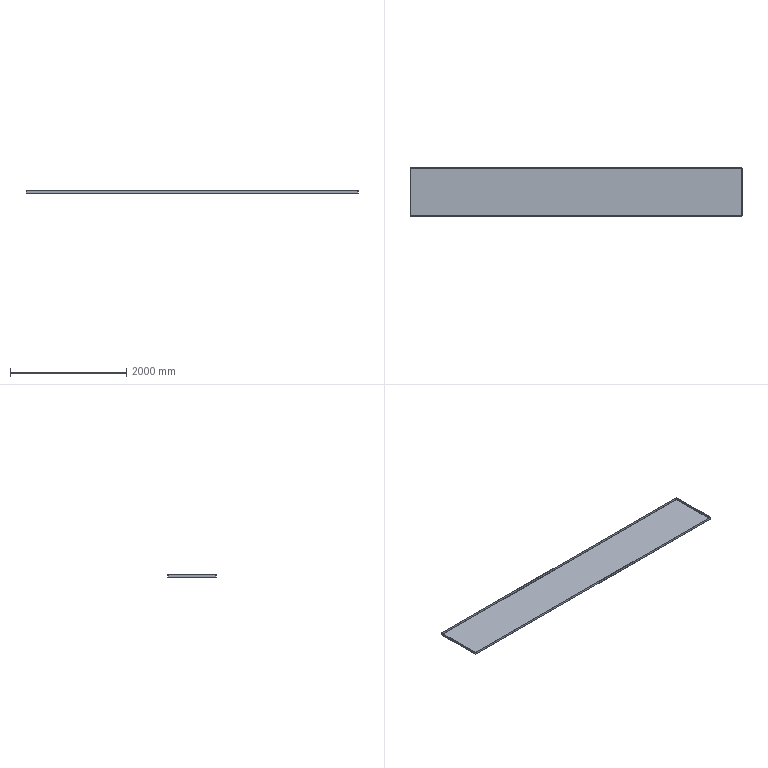Part | SolidWorks | features EdgeFlange 1, FlatPattern 1, SMBaseFlange 1, SheetMetal 1 | 1 solid | 38 faces | box 5700 x 825 x 40 mm | volume 10375674 mm3 | plane 22 | spline 8 | cylinder 8 | commonest cylinder face diameters 1.473 x4 5.473 x4
STEP:
#1=CARTESIAN_POINT('',(2847.263,409.763,-2.));
#2=VERTEX_POINT('',#1);
#3=CARTESIAN_POINT('',(2847.263,-409.763,-2.));
#4=VERTEX_POINT('',#3);
#5=CARTESIAN_POINT('',(2847.263,409.793,-2.));
#6=DIRECTION('',(0.,-1.,0.));
#7=VECTOR('',#6,1000.);
#8=LINE('',#5,#7);
#9=EDGE_CURVE('',#2,#4,#8,.T.);
#10=ORIENTED_EDGE('',*,*,#9,.T.);
#11=CARTESIAN_POINT('',(-2847.263,-409.763,-2.));
#12=VERTEX_POINT('',#11);
#13=CARTESIAN_POINT('',(2847.293,-409.763,-2.));
#14=DIRECTION('',(-1.,0.,0.));
#15=VECTOR('',#14,1000.);
#16=LINE('',#13,#15);
#17=EDGE_CURVE('',#4,#12,#16,.T.);
#18=ORIENTED_EDGE('',*,*,#17,.T.);
#19=CARTESIAN_POINT('',(-2847.263,409.763,-2.));
#20=VERTEX_POINT('',#19);
#21=CARTESIAN_POINT('',(-2847.263,-409.793,-2.));
#22=DIRECTION('',(0.,1.,0.));
#23=VECTOR('',#22,1000.);
#24=LINE('',#21,#23);
#25=EDGE_CURVE('',#12,#20,#24,.T.);
#26=ORIENTED_EDGE('',*,*,#25,.T.);
#27=CARTESIAN_POINT('',(-2847.293,409.763,-2.));
#28=DIRECTION('',(1.,0.,0.));
#29=VECTOR('',#28,1000.);
#30=LINE('',#27,#29);
#31=EDGE_CURVE('',#20,#2,#30,.T.);
#32=ORIENTED_EDGE('',*,*,#31,.T.);
#33=EDGE_LOOP('',(#10,#18,#26,#32));
#34=FACE_OUTER_BOUND('',#33,.T.);
#35=CARTESIAN_POINT('',(0.,0.,-2.));
#36=DIRECTION('',(0.,0.,-1.));
#37=DIRECTION('',(-1.,0.,0.));
#38=AXIS2_PLACEMENT_3D('',#35,#36,#37);
#39=PLANE('',#38);
#40=ADVANCED_FACE('',(#34),#39,.T.);
#41=CARTESIAN_POINT('',(2847.263,-409.763,0.));
#42=VERTEX_POINT('',#41);
#43=CARTESIAN_POINT('',(-2847.263,-409.763,0.));
#44=VERTEX_POINT('',#43);
#45=CARTESIAN_POINT('',(2847.293,-409.763,0.));
#46=DIRECTION('',(-1.,0.,0.));
#47=VECTOR('',#46,1000.);
#48=LINE('',#45,#47);
#49=EDGE_CURVE('',#42,#44,#48,.T.);
#50=ORIENTED_EDGE('',*,*,#49,.F.);
#51=CARTESIAN_POINT('',(2847.263,409.763,0.));
#52=VERTEX_POINT('',#51);
#53=CARTESIAN_POINT('',(2847.263,409.793,0.));
#54=DIRECTION('',(0.,-1.,0.));
#55=VECTOR('',#54,1000.);
#56=LINE('',#53,#55);
#57=EDGE_CURVE('',#52,#42,#56,.T.);
#58=ORIENTED_EDGE('',*,*,#57,.F.);
#59=CARTESIAN_POINT('',(-2847.263,409.763,0.));
#60=VERTEX_POINT('',#59);
#61=CARTESIAN_POINT('',(-2847.293,409.763,0.));
#62=DIRECTION('',(1.,0.,0.));
#63=VECTOR('',#62,1000.);
#64=LINE('',#61,#63);
#65=EDGE_CURVE('',#60,#52,#64,.T.);
#66=ORIENTED_EDGE('',*,*,#65,.F.);
#67=CARTESIAN_POINT('',(-2847.263,-409.793,0.));
#68=DIRECTION('',(0.,1.,0.));
#69=VECTOR('',#68,1000.);
#70=LINE('',#67,#69);
#71=EDGE_CURVE('',#44,#60,#70,.T.);
#72=ORIENTED_EDGE('',*,*,#71,.F.);
#73=EDGE_LOOP('',(#50,#58,#66,#72));
#74=FACE_OUTER_BOUND('',#73,.T.);
#75=CARTESIAN_POINT('',(0.,0.,0.));
#76=DIRECTION('',(0.,0.,-1.));
#77=DIRECTION('',(-1.,0.,0.));
#78=AXIS2_PLACEMENT_3D('',#75,#76,#77);
#79=PLANE('',#78);
#80=ADVANCED_FACE('',(#74),#79,.F.);
#81=CARTESIAN_POINT('',(2847.293,412.5,0.7366));
#82=VERTEX_POINT('',#81);
#83=CARTESIAN_POINT('',(2847.293,410.5,0.7366));
#84=VERTEX_POINT('',#83);
#85=CARTESIAN_POINT('',(2847.293,410.5,0.7366));
#86=DIRECTION('',(0.,-1.,0.));
#87=VECTOR('',#86,1000.);
#88=LINE('',#85,#87);
#89=EDGE_CURVE('',#82,#84,#88,.T.);
#90=ORIENTED_EDGE('',*,*,#89,.T.);
#91=CARTESIAN_POINT('',(2847.263,409.763,0.));
#92=CARTESIAN_POINT('',(2847.268,409.956,0.));
#93=CARTESIAN_POINT('',(2847.273,410.148,0.07939));
#94=CARTESIAN_POINT('',(2847.283,410.421,0.3521));
#95=CARTESIAN_POINT('',(2847.288,410.5,0.5438));
#96=CARTESIAN_POINT('',(2847.293,410.5,0.7366));
#97=B_SPLINE_CURVE_WITH_KNOTS('',3,(#91,#92,#93,#94,#95,#96),.UNSPECIFIED.,.F.,.F.,(4,2,4),(0.,0.5,1.),.UNSPECIFIED.);
#98=EDGE_CURVE('',#52,#84,#97,.T.);
#99=ORIENTED_EDGE('',*,*,#98,.F.);
#100=CARTESIAN_POINT('',(2847.263,409.763,0.));
#101=DIRECTION('',(0.,0.,-1.));
#102=VECTOR('',#101,1000.);
#103=LINE('',#100,#102);
#104=EDGE_CURVE('',#52,#2,#103,.T.);
#105=ORIENTED_EDGE('',*,*,#104,.T.);
#106=CARTESIAN_POINT('',(2847.263,409.763,-2.));
#107=CARTESIAN_POINT('',(2847.266,410.122,-2.));
#108=CARTESIAN_POINT('',(2847.268,410.48,-1.929));
#109=CARTESIAN_POINT('',(2847.273,411.142,-1.655));
#110=CARTESIAN_POINT('',(2847.276,411.445,-1.452));
#111=CARTESIAN_POINT('',(2847.281,411.952,-0.9452));
#112=CARTESIAN_POINT('',(2847.283,412.155,-0.6416));
#113=CARTESIAN_POINT('',(2847.288,412.429,0.0203));
#114=CARTESIAN_POINT('',(2847.29,412.5,0.3784));
#115=CARTESIAN_POINT('',(2847.293,412.5,0.7366));
#116=B_SPLINE_CURVE_WITH_KNOTS('',3,(#106,#107,#108,#109,#110,#111,#112,#113,#114,#115),.UNSPECIFIED.,.F.,.F.,(4,2,2,2,4),(0.,0.25,0.5,0.75,1.),.UNSPECIFIED.);
#117=EDGE_CURVE('',#2,#82,#116,.T.);
#118=ORIENTED_EDGE('',*,*,#117,.T.);
#119=EDGE_LOOP('',(#90,#99,#105,#118));
#120=FACE_OUTER_BOUND('',#119,.T.);
#121=CARTESIAN_POINT('',(2847.263,409.763,-2.02));
#122=CARTESIAN_POINT('',(2847.266,410.124,-2.02));
#123=CARTESIAN_POINT('',(2847.268,410.485,-1.948));
#124=CARTESIAN_POINT('',(2847.273,411.152,-1.672));
#125=CARTESIAN_POINT('',(2847.276,411.457,-1.468));
#126=CARTESIAN_POINT('',(2847.281,411.968,-0.9575));
#127=CARTESIAN_POINT('',(2847.283,412.172,-0.6517));
#128=CARTESIAN_POINT('',(2847.288,412.448,0.01507));
#129=CARTESIAN_POINT('',(2847.29,412.52,0.3757));
#130=CARTESIAN_POINT('',(2847.293,412.52,0.7366));
#131=CARTESIAN_POINT('',(2847.263,409.763,-2.));
#132=CARTESIAN_POINT('',(2847.266,410.122,-2.));
#133=CARTESIAN_POINT('',(2847.268,410.48,-1.929));
#134=CARTESIAN_POINT('',(2847.273,411.142,-1.655));
#135=CARTESIAN_POINT('',(2847.276,411.445,-1.452));
#136=CARTESIAN_POINT('',(2847.281,411.952,-0.9452));
#137=CARTESIAN_POINT('',(2847.283,412.155,-0.6416));
#138=CARTESIAN_POINT('',(2847.288,412.429,0.0203));
#139=CARTESIAN_POINT('',(2847.29,412.5,0.3783));
#140=CARTESIAN_POINT('',(2847.293,412.5,0.7366));
#141=CARTESIAN_POINT('',(2847.263,409.763,0.));
#142=CARTESIAN_POINT('',(2847.266,409.86,0.));
#143=CARTESIAN_POINT('',(2847.268,409.956,0.01917));
#144=CARTESIAN_POINT('',(2847.273,410.134,0.09297));
#145=CARTESIAN_POINT('',(2847.276,410.216,0.1476));
#146=CARTESIAN_POINT('',(2847.281,410.352,0.2839));
#147=CARTESIAN_POINT('',(2847.283,410.407,0.3656));
#148=CARTESIAN_POINT('',(2847.288,410.481,0.5438));
#149=CARTESIAN_POINT('',(2847.29,410.5,0.6402));
#150=CARTESIAN_POINT('',(2847.293,410.5,0.7366));
#151=CARTESIAN_POINT('',(2847.263,409.763,0.0202));
#152=CARTESIAN_POINT('',(2847.266,409.857,0.0202));
#153=CARTESIAN_POINT('',(2847.268,409.951,0.03885));
#154=CARTESIAN_POINT('',(2847.273,410.124,0.1106));
#155=CARTESIAN_POINT('',(2847.276,410.204,0.1637));
#156=CARTESIAN_POINT('',(2847.281,410.336,0.2963));
#157=CARTESIAN_POINT('',(2847.283,410.389,0.3758));
#158=CARTESIAN_POINT('',(2847.288,410.461,0.5491));
#159=CARTESIAN_POINT('',(2847.29,410.48,0.6428));
#160=CARTESIAN_POINT('',(2847.293,410.48,0.7366));
#161=B_SPLINE_SURFACE_WITH_KNOTS('',1,3,((#121,#122,#123,#124,#125,#126,#127,#128,#129,#130),(#131,#132,#133,#134,#135,#136,#137,#138,#139,#140),(#141,#142,#143,#144,#145,#146,#147,#148,#149,#150),(#151,#152,#153,#154,#155,#156,#157,#158,#159,#160)),.UNSPECIFIED.,.F.,.F.,.F.,(2,1,1,2),(4,2,2,2,4),(-0.01,0.,1.,1.01),(0.,0.25,0.5,0.75,1.),.UNSPECIFIED.);
#162=ADVANCED_FACE('',(#120),#161,.F.);
#163=CARTESIAN_POINT('',(-2847.293,410.5,0.7366));
#164=VERTEX_POINT('',#163);
#165=CARTESIAN_POINT('',(-2847.293,410.5,0.7366));
#166=CARTESIAN_POINT('',(-2847.288,410.5,0.5438));
#167=CARTESIAN_POINT('',(-2847.283,410.421,0.3521));
#168=CARTESIAN_POINT('',(-2847.273,410.148,0.07939));
#169=CARTESIAN_POINT('',(-2847.268,409.956,0.));
#170=CARTESIAN_POINT('',(-2847.263,409.763,0.));
#171=B_SPLINE_CURVE_WITH_KNOTS('',3,(#165,#166,#167,#168,#169,#170),.UNSPECIFIED.,.F.,.F.,(4,2,4),(0.,0.5,1.),.UNSPECIFIED.);
#172=EDGE_CURVE('',#164,#60,#171,.T.);
#173=ORIENTED_EDGE('',*,*,#172,.F.);
#174=CARTESIAN_POINT('',(-2847.293,412.5,0.7366));
#175=VERTEX_POINT('',#174);
#176=CARTESIAN_POINT('',(-2847.293,410.5,0.7366));
#177=DIRECTION('',(0.,-1.,0.));
#178=VECTOR('',#177,1000.);
#179=LINE('',#176,#178);
#180=EDGE_CURVE('',#175,#164,#179,.T.);
#181=ORIENTED_EDGE('',*,*,#180,.F.);
#182=CARTESIAN_POINT('',(-2847.293,412.5,0.7366));
#183=CARTESIAN_POINT('',(-2847.29,412.5,0.3784));
#184=CARTESIAN_POINT('',(-2847.288,412.429,0.0203));
#185=CARTESIAN_POINT('',(-2847.283,412.155,-0.6416));
#186=CARTESIAN_POINT('',(-2847.281,411.952,-0.9452));
#187=CARTESIAN_POINT('',(-2847.276,411.445,-1.452));
#188=CARTESIAN_POINT('',(-2847.273,411.142,-1.655));
#189=CARTESIAN_POINT('',(-2847.268,410.48,-1.929));
#190=CARTESIAN_POINT('',(-2847.266,410.122,-2.));
#191=CARTESIAN_POINT('',(-2847.263,409.763,-2.));
#192=B_SPLINE_CURVE_WITH_KNOTS('',3,(#182,#183,#184,#185,#186,#187,#188,#189,#190,#191),.UNSPECIFIED.,.F.,.F.,(4,2,2,2,4),(0.,0.25,0.5,0.75,1.),.UNSPECIFIED.);
#193=EDGE_CURVE('',#175,#20,#192,.T.);
#194=ORIENTED_EDGE('',*,*,#193,.T.);
#195=CARTESIAN_POINT('',(-2847.263,409.763,0.));
#196=DIRECTION('',(0.,0.,-1.));
#197=VECTOR('',#196,1000.);
#198=LINE('',#195,#197);
#199=EDGE_CURVE('',#60,#20,#198,.T.);
#200=ORIENTED_EDGE('',*,*,#199,.F.);
#201=EDGE_LOOP('',(#173,#181,#194,#200));
#202=FACE_OUTER_BOUND('',#201,.T.);
#203=CARTESIAN_POINT('',(-2847.293,412.52,0.7366));
#204=CARTESIAN_POINT('',(-2847.29,412.52,0.3757));
#205=CARTESIAN_POINT('',(-2847.288,412.448,0.01507));
#206=CARTESIAN_POINT('',(-2847.283,412.172,-0.6517));
#207=CARTESIAN_POINT('',(-2847.281,411.968,-0.9575));
#208=CARTESIAN_POINT('',(-2847.276,411.457,-1.468));
#209=CARTESIAN_POINT('',(-2847.273,411.152,-1.672));
#210=CARTESIAN_POINT('',(-2847.268,410.485,-1.948));
#211=CARTESIAN_POINT('',(-2847.266,410.124,-2.02));
#212=CARTESIAN_POINT('',(-2847.263,409.763,-2.02));
#213=CARTESIAN_POINT('',(-2847.293,412.5,0.7366));
#214=CARTESIAN_POINT('',(-2847.29,412.5,0.3783));
#215=CARTESIAN_POINT('',(-2847.288,412.429,0.0203));
#216=CARTESIAN_POINT('',(-2847.283,412.155,-0.6416));
#217=CARTESIAN_POINT('',(-2847.281,411.952,-0.9452));
#218=CARTESIAN_POINT('',(-2847.276,411.445,-1.452));
#219=CARTESIAN_POINT('',(-2847.273,411.142,-1.655));
#220=CARTESIAN_POINT('',(-2847.268,410.48,-1.929));
#221=CARTESIAN_POINT('',(-2847.266,410.122,-2.));
#222=CARTESIAN_POINT('',(-2847.263,409.763,-2.));
#223=CARTESIAN_POINT('',(-2847.293,410.5,0.7366));
#224=CARTESIAN_POINT('',(-2847.29,410.5,0.6402));
#225=CARTESIAN_POINT('',(-2847.288,410.481,0.5438));
#226=CARTESIAN_POINT('',(-2847.283,410.407,0.3656));
#227=CARTESIAN_POINT('',(-2847.281,410.352,0.2839));
#228=CARTESIAN_POINT('',(-2847.276,410.216,0.1476));
#229=CARTESIAN_POINT('',(-2847.273,410.134,0.09297));
#230=CARTESIAN_POINT('',(-2847.268,409.956,0.01917));
#231=CARTESIAN_POINT('',(-2847.266,409.86,0.));
#232=CARTESIAN_POINT('',(-2847.263,409.763,0.));
#233=CARTESIAN_POINT('',(-2847.293,410.48,0.7366));
#234=CARTESIAN_POINT('',(-2847.29,410.48,0.6428));
#235=CARTESIAN_POINT('',(-2847.288,410.461,0.5491));
#236=CARTESIAN_POINT('',(-2847.283,410.389,0.3758));
#237=CARTESIAN_POINT('',(-2847.281,410.336,0.2963));
#238=CARTESIAN_POINT('',(-2847.276,410.204,0.1637));
#239=CARTESIAN_POINT('',(-2847.273,410.124,0.1106));
#240=CARTESIAN_POINT('',(-2847.268,409.951,0.03885));
#241=CARTESIAN_POINT('',(-2847.266,409.857,0.0202));
#242=CARTESIAN_POINT('',(-2847.263,409.763,0.0202));
#243=B_SPLINE_SURFACE_WITH_KNOTS('',1,3,((#203,#204,#205,#206,#207,#208,#209,#210,#211,#212),(#213,#214,#215,#216,#217,#218,#219,#220,#221,#222),(#223,#224,#225,#226,#227,#228,#229,#230,#231,#232),(#233,#234,#235,#236,#237,#238,#239,#240,#241,#242)),.UNSPECIFIED.,.F.,.F.,.F.,(2,1,1,2),(4,2,2,2,4),(-0.01,0.,1.,1.01),(0.,0.25,0.5,0.75,1.),.UNSPECIFIED.);
#244=ADVANCED_FACE('',(#202),#243,.F.);
#245=ORIENTED_EDGE('',*,*,#31,.F.);
#246=ORIENTED_EDGE('',*,*,#193,.F.);
#247=CARTESIAN_POINT('',(0.,412.5,0.7366));
#248=DIRECTION('',(-1.,0.,0.));
#249=VECTOR('',#248,1000.);
#250=LINE('',#247,#249);
#251=EDGE_CURVE('',#82,#175,#250,.T.);
#252=ORIENTED_EDGE('',*,*,#251,.F.);
#253=ORIENTED_EDGE('',*,*,#117,.F.);
#254=EDGE_LOOP('',(#245,#246,#252,#253));
#255=FACE_OUTER_BOUND('',#254,.T.);
#256=CARTESIAN_POINT('',(-2847.293,409.763,0.7366));
#257=DIRECTION('',(-1.,0.,0.));
#258=DIRECTION('',(0.,1.,0.));
#259=AXIS2_PLACEMENT_3D('',#256,#257,#258);
#260=CYLINDRICAL_SURFACE('',#259,2.737);
#261=ADVANCED_FACE('',(#255),#260,.T.);
#262=ORIENTED_EDGE('',*,*,#65,.T.);
#263=ORIENTED_EDGE('',*,*,#98,.T.);
#264=CARTESIAN_POINT('',(2850.,410.5,0.7366));
#265=DIRECTION('',(-1.,0.,0.));
#266=VECTOR('',#265,1000.);
#267=LINE('',#264,#266);
#268=EDGE_CURVE('',#84,#164,#267,.T.);
#269=ORIENTED_EDGE('',*,*,#268,.T.);
#270=ORIENTED_EDGE('',*,*,#172,.T.);
#271=EDGE_LOOP('',(#262,#263,#269,#270));
#272=FACE_OUTER_BOUND('',#271,.T.);
#273=CARTESIAN_POINT('',(-2847.293,409.763,0.7366));
#274=DIRECTION('',(-1.,0.,0.));
#275=DIRECTION('',(0.,1.,0.));
#276=AXIS2_PLACEMENT_3D('',#273,#274,#275);
#277=CYLINDRICAL_SURFACE('',#276,0.7366);
#278=ADVANCED_FACE('',(#272),#277,.F.);
#279=CARTESIAN_POINT('',(2847.293,410.5,38.));
#280=VERTEX_POINT('',#279);
#281=CARTESIAN_POINT('',(2847.293,412.5,38.));
#282=VERTEX_POINT('',#281);
#283=CARTESIAN_POINT('',(2847.293,412.5,38.));
#284=DIRECTION('',(0.,1.,0.));
#285=VECTOR('',#284,1000.);
#286=LINE('',#283,#285);
#287=EDGE_CURVE('',#280,#282,#286,.T.);
#288=ORIENTED_EDGE('',*,*,#287,.F.);
#289=CARTESIAN_POINT('',(2847.293,410.5,0.));
#290=DIRECTION('',(0.,0.,1.));
#291=VECTOR('',#290,1000.);
#292=LINE('',#289,#291);
#293=EDGE_CURVE('',#84,#280,#292,.T.);
#294=ORIENTED_EDGE('',*,*,#293,.F.);
#295=ORIENTED_EDGE('',*,*,#89,.F.);
#296=CARTESIAN_POINT('',(2847.293,412.5,0.));
#297=DIRECTION('',(0.,0.,-1.));
#298=VECTOR('',#297,1000.);
#299=LINE('',#296,#298);
#300=EDGE_CURVE('',#282,#82,#299,.T.);
#301=ORIENTED_EDGE('',*,*,#300,.F.);
#302=EDGE_LOOP('',(#288,#294,#295,#301));
#303=FACE_OUTER_BOUND('',#302,.T.);
#304=CARTESIAN_POINT('',(2847.293,410.5,0.));
#305=DIRECTION('',(1.,0.,0.));
#306=DIRECTION('',(0.,0.,-1.));
#307=AXIS2_PLACEMENT_3D('',#304,#305,#306);
#308=PLANE('',#307);
#309=ADVANCED_FACE('',(#303),#308,.T.);
#310=CARTESIAN_POINT('',(-2847.293,412.5,38.));
#311=VERTEX_POINT('',#310);
#312=CARTESIAN_POINT('',(-2847.293,412.5,0.));
#313=DIRECTION('',(0.,0.,-1.));
#314=VECTOR('',#313,1000.);
#315=LINE('',#312,#314);
#316=EDGE_CURVE('',#311,#175,#315,.T.);
#317=ORIENTED_EDGE('',*,*,#316,.F.);
#318=CARTESIAN_POINT('',(-2850.,412.5,38.));
#319=DIRECTION('',(-1.,0.,0.));
#320=VECTOR('',#319,1000.);
#321=LINE('',#318,#320);
#322=EDGE_CURVE('',#282,#311,#321,.T.);
#323=ORIENTED_EDGE('',*,*,#322,.F.);
#324=ORIENTED_EDGE('',*,*,#300,.T.);
#325=ORIENTED_EDGE('',*,*,#251,.T.);
#326=EDGE_LOOP('',(#317,#323,#324,#325));
#327=FACE_OUTER_BOUND('',#326,.T.);
#328=CARTESIAN_POINT('',(0.,412.5,0.));
#329=DIRECTION('',(0.,1.,0.));
#330=DIRECTION('',(0.,0.,1.));
#331=AXIS2_PLACEMENT_3D('',#328,#329,#330);
#332=PLANE('',#331);
#333=ADVANCED_FACE('',(#327),#332,.T.);
#334=CARTESIAN_POINT('',(-2847.293,410.5,38.));
#335=VERTEX_POINT('',#334);
#336=CARTESIAN_POINT('',(0.,410.5,38.));
#337=DIRECTION('',(-1.,0.,0.));
#338=VECTOR('',#337,1000.);
#339=LINE('',#336,#338);
#340=EDGE_CURVE('',#280,#335,#339,.T.);
#341=ORIENTED_EDGE('',*,*,#340,.T.);
#342=CARTESIAN_POINT('',(-2847.293,410.5,0.));
#343=DIRECTION('',(0.,0.,1.));
#344=VECTOR('',#343,1000.);
#345=LINE('',#342,#344);
#346=EDGE_CURVE('',#164,#335,#345,.T.);
#347=ORIENTED_EDGE('',*,*,#346,.F.);
#348=ORIENTED_EDGE('',*,*,#268,.F.);
#349=ORIENTED_EDGE('',*,*,#293,.T.);
#350=EDGE_LOOP('',(#341,#347,#348,#349));
#351=FACE_OUTER_BOUND('',#350,.T.);
#352=CARTESIAN_POINT('',(0.,410.5,0.));
#353=DIRECTION('',(0.,1.,0.));
#354=DIRECTION('',(0.,0.,1.));
#355=AXIS2_PLACEMENT_3D('',#352,#353,#354);
#356=PLANE('',#355);
#357=ADVANCED_FACE('',(#351),#356,.F.);
#358=CARTESIAN_POINT('',(-2847.293,410.5,38.));
#359=DIRECTION('',(0.,1.,0.));
#360=VECTOR('',#359,1000.);
#361=LINE('',#358,#360);
#362=EDGE_CURVE('',#335,#311,#361,.T.);
#363=ORIENTED_EDGE('',*,*,#362,.F.);
#364=ORIENTED_EDGE('',*,*,#340,.F.);
#365=ORIENTED_EDGE('',*,*,#287,.T.);
#366=ORIENTED_EDGE('',*,*,#322,.T.);
#367=EDGE_LOOP('',(#363,#364,#365,#366));
#368=FACE_OUTER_BOUND('',#367,.T.);
#369=CARTESIAN_POINT('',(-2850.,412.5,38.));
#370=DIRECTION('',(0.,0.,1.));
#371=DIRECTION('',(0.,-1.,0.));
#372=AXIS2_PLACEMENT_3D('',#369,#370,#371);
#373=PLANE('',#372);
#374=ADVANCED_FACE('',(#368),#373,.T.);
#375=ORIENTED_EDGE('',*,*,#346,.T.);
#376=ORIENTED_EDGE('',*,*,#362,.T.);
#377=ORIENTED_EDGE('',*,*,#316,.T.);
#378=ORIENTED_EDGE('',*,*,#180,.T.);
#379=EDGE_LOOP('',(#375,#376,#377,#378));
#380=FACE_OUTER_BOUND('',#379,.T.);
#381=CARTESIAN_POINT('',(-2847.293,410.5,0.));
#382=DIRECTION('',(1.,0.,0.));
#383=DIRECTION('',(0.,0.,-1.));
#384=AXIS2_PLACEMENT_3D('',#381,#382,#383);
#385=PLANE('',#384);
#386=ADVANCED_FACE('',(#380),#385,.F.);
#387=CARTESIAN_POINT('',(-2850.,409.793,0.7366));
#388=VERTEX_POINT('',#387);
#389=CARTESIAN_POINT('',(-2848.,409.793,0.7366));
#390=VERTEX_POINT('',#389);
#391=CARTESIAN_POINT('',(-2848.,409.793,0.7366));
#392=DIRECTION('',(1.,0.,0.));
#393=VECTOR('',#392,1000.);
#394=LINE('',#391,#393);
#395=EDGE_CURVE('',#388,#390,#394,.T.);
#396=ORIENTED_EDGE('',*,*,#395,.T.);
#397=CARTESIAN_POINT('',(-2847.263,409.763,0.));
#398=CARTESIAN_POINT('',(-2847.456,409.768,0.));
#399=CARTESIAN_POINT('',(-2847.648,409.773,0.07939));
#400=CARTESIAN_POINT('',(-2847.921,409.783,0.3521));
#401=CARTESIAN_POINT('',(-2848.,409.788,0.5438));
#402=CARTESIAN_POINT('',(-2848.,409.793,0.7366));
#403=B_SPLINE_CURVE_WITH_KNOTS('',3,(#397,#398,#399,#400,#401,#402),.UNSPECIFIED.,.F.,.F.,(4,2,4),(0.,0.5,1.),.UNSPECIFIED.);
#404=EDGE_CURVE('',#60,#390,#403,.T.);
#405=ORIENTED_EDGE('',*,*,#404,.F.);
#406=ORIENTED_EDGE('',*,*,#199,.T.);
#407=CARTESIAN_POINT('',(-2847.263,409.763,-2.));
#408=CARTESIAN_POINT('',(-2847.622,409.766,-2.));
#409=CARTESIAN_POINT('',(-2847.98,409.768,-1.929));
#410=CARTESIAN_POINT('',(-2848.642,409.773,-1.655));
#411=CARTESIAN_POINT('',(-2848.945,409.776,-1.452));
#412=CARTESIAN_POINT('',(-2849.452,409.781,-0.9452));
#413=CARTESIAN_POINT('',(-2849.655,409.783,-0.6416));
#414=CARTESIAN_POINT('',(-2849.929,409.788,0.0203));
#415=CARTESIAN_POINT('',(-2850.,409.79,0.3784));
#416=CARTESIAN_POINT('',(-2850.,409.793,0.7366));
#417=B_SPLINE_CURVE_WITH_KNOTS('',3,(#407,#408,#409,#410,#411,#412,#413,#414,#415,#416),.UNSPECIFIED.,.F.,.F.,(4,2,2,2,4),(0.,0.25,0.5,0.75,1.),.UNSPECIFIED.);
#418=EDGE_CURVE('',#20,#388,#417,.T.);
#419=ORIENTED_EDGE('',*,*,#418,.T.);
#420=EDGE_LOOP('',(#396,#405,#406,#419));
#421=FACE_OUTER_BOUND('',#420,.T.);
#422=CARTESIAN_POINT('',(-2847.263,409.763,-2.02));
#423=CARTESIAN_POINT('',(-2847.624,409.766,-2.02));
#424=CARTESIAN_POINT('',(-2847.985,409.768,-1.948));
#425=CARTESIAN_POINT('',(-2848.652,409.773,-1.672));
#426=CARTESIAN_POINT('',(-2848.957,409.776,-1.468));
#427=CARTESIAN_POINT('',(-2849.468,409.781,-0.9575));
#428=CARTESIAN_POINT('',(-2849.672,409.783,-0.6517));
#429=CARTESIAN_POINT('',(-2849.948,409.788,0.01507));
#430=CARTESIAN_POINT('',(-2850.02,409.79,0.3757));
#431=CARTESIAN_POINT('',(-2850.02,409.793,0.7366));
#432=CARTESIAN_POINT('',(-2847.263,409.763,-2.));
#433=CARTESIAN_POINT('',(-2847.622,409.766,-2.));
#434=CARTESIAN_POINT('',(-2847.98,409.768,-1.929));
#435=CARTESIAN_POINT('',(-2848.642,409.773,-1.655));
#436=CARTESIAN_POINT('',(-2848.945,409.776,-1.452));
#437=CARTESIAN_POINT('',(-2849.452,409.781,-0.9452));
#438=CARTESIAN_POINT('',(-2849.655,409.783,-0.6416));
#439=CARTESIAN_POINT('',(-2849.929,409.788,0.0203));
#440=CARTESIAN_POINT('',(-2850.,409.79,0.3783));
#441=CARTESIAN_POINT('',(-2850.,409.793,0.7366));
#442=CARTESIAN_POINT('',(-2847.263,409.763,0.));
#443=CARTESIAN_POINT('',(-2847.36,409.766,0.));
#444=CARTESIAN_POINT('',(-2847.456,409.768,0.01917));
#445=CARTESIAN_POINT('',(-2847.634,409.773,0.09297));
#446=CARTESIAN_POINT('',(-2847.716,409.776,0.1476));
#447=CARTESIAN_POINT('',(-2847.852,409.781,0.2839));
#448=CARTESIAN_POINT('',(-2847.907,409.783,0.3656));
#449=CARTESIAN_POINT('',(-2847.981,409.788,0.5438));
#450=CARTESIAN_POINT('',(-2848.,409.79,0.6402));
#451=CARTESIAN_POINT('',(-2848.,409.793,0.7366));
#452=CARTESIAN_POINT('',(-2847.263,409.763,0.0202));
#453=CARTESIAN_POINT('',(-2847.357,409.766,0.0202));
#454=CARTESIAN_POINT('',(-2847.451,409.768,0.03885));
#455=CARTESIAN_POINT('',(-2847.624,409.773,0.1106));
#456=CARTESIAN_POINT('',(-2847.704,409.776,0.1637));
#457=CARTESIAN_POINT('',(-2847.836,409.781,0.2963));
#458=CARTESIAN_POINT('',(-2847.889,409.783,0.3758));
#459=CARTESIAN_POINT('',(-2847.961,409.788,0.5491));
#460=CARTESIAN_POINT('',(-2847.98,409.79,0.6428));
#461=CARTESIAN_POINT('',(-2847.98,409.793,0.7366));
#462=B_SPLINE_SURFACE_WITH_KNOTS('',1,3,((#422,#423,#424,#425,#426,#427,#428,#429,#430,#431),(#432,#433,#434,#435,#436,#437,#438,#439,#440,#441),(#442,#443,#444,#445,#446,#447,#448,#449,#450,#451),(#452,#453,#454,#455,#456,#457,#458,#459,#460,#461)),.UNSPECIFIED.,.F.,.F.,.F.,(2,1,1,2),(4,2,2,2,4),(-0.01,0.,1.,1.01),(0.,0.25,0.5,0.75,1.),.UNSPECIFIED.);
#463=ADVANCED_FACE('',(#421),#462,.F.);
#464=CARTESIAN_POINT('',(-2848.,-409.793,0.7366));
#465=VERTEX_POINT('',#464);
#466=CARTESIAN_POINT('',(-2848.,-409.793,0.7366));
#467=CARTESIAN_POINT('',(-2848.,-409.788,0.5438));
#468=CARTESIAN_POINT('',(-2847.921,-409.783,0.3521));
#469=CARTESIAN_POINT('',(-2847.648,-409.773,0.07939));
#470=CARTESIAN_POINT('',(-2847.456,-409.768,0.));
#471=CARTESIAN_POINT('',(-2847.263,-409.763,0.));
#472=B_SPLINE_CURVE_WITH_KNOTS('',3,(#466,#467,#468,#469,#470,#471),.UNSPECIFIED.,.F.,.F.,(4,2,4),(0.,0.5,1.),.UNSPECIFIED.);
#473=EDGE_CURVE('',#465,#44,#472,.T.);
#474=ORIENTED_EDGE('',*,*,#473,.F.);
#475=CARTESIAN_POINT('',(-2850.,-409.793,0.7366));
#476=VERTEX_POINT('',#475);
#477=CARTESIAN_POINT('',(-2848.,-409.793,0.7366));
#478=DIRECTION('',(1.,0.,0.));
#479=VECTOR('',#478,1000.);
#480=LINE('',#477,#479);
#481=EDGE_CURVE('',#476,#465,#480,.T.);
#482=ORIENTED_EDGE('',*,*,#481,.F.);
#483=CARTESIAN_POINT('',(-2850.,-409.793,0.7366));
#484=CARTESIAN_POINT('',(-2850.,-409.79,0.3784));
#485=CARTESIAN_POINT('',(-2849.929,-409.788,0.0203));
#486=CARTESIAN_POINT('',(-2849.655,-409.783,-0.6416));
#487=CARTESIAN_POINT('',(-2849.452,-409.781,-0.9452));
#488=CARTESIAN_POINT('',(-2848.945,-409.776,-1.452));
#489=CARTESIAN_POINT('',(-2848.642,-409.773,-1.655));
#490=CARTESIAN_POINT('',(-2847.98,-409.768,-1.929));
#491=CARTESIAN_POINT('',(-2847.622,-409.766,-2.));
#492=CARTESIAN_POINT('',(-2847.263,-409.763,-2.));
#493=B_SPLINE_CURVE_WITH_KNOTS('',3,(#483,#484,#485,#486,#487,#488,#489,#490,#491,#492),.UNSPECIFIED.,.F.,.F.,(4,2,2,2,4),(0.,0.25,0.5,0.75,1.),.UNSPECIFIED.);
#494=EDGE_CURVE('',#476,#12,#493,.T.);
#495=ORIENTED_EDGE('',*,*,#494,.T.);
#496=CARTESIAN_POINT('',(-2847.263,-409.763,0.));
#497=DIRECTION('',(0.,0.,-1.));
#498=VECTOR('',#497,1000.);
#499=LINE('',#496,#498);
#500=EDGE_CURVE('',#44,#12,#499,.T.);
#501=ORIENTED_EDGE('',*,*,#500,.F.);
#502=EDGE_LOOP('',(#474,#482,#495,#501));
#503=FACE_OUTER_BOUND('',#502,.T.);
#504=CARTESIAN_POINT('',(-2850.02,-409.793,0.7366));
#505=CARTESIAN_POINT('',(-2850.02,-409.79,0.3757));
#506=CARTESIAN_POINT('',(-2849.948,-409.788,0.01507));
#507=CARTESIAN_POINT('',(-2849.672,-409.783,-0.6517));
#508=CARTESIAN_POINT('',(-2849.468,-409.781,-0.9575));
#509=CARTESIAN_POINT('',(-2848.957,-409.776,-1.468));
#510=CARTESIAN_POINT('',(-2848.652,-409.773,-1.672));
#511=CARTESIAN_POINT('',(-2847.985,-409.768,-1.948));
#512=CARTESIAN_POINT('',(-2847.624,-409.766,-2.02));
#513=CARTESIAN_POINT('',(-2847.263,-409.763,-2.02));
#514=CARTESIAN_POINT('',(-2850.,-409.793,0.7366));
#515=CARTESIAN_POINT('',(-2850.,-409.79,0.3783));
#516=CARTESIAN_POINT('',(-2849.929,-409.788,0.0203));
#517=CARTESIAN_POINT('',(-2849.655,-409.783,-0.6416));
#518=CARTESIAN_POINT('',(-2849.452,-409.781,-0.9452));
#519=CARTESIAN_POINT('',(-2848.945,-409.776,-1.452));
#520=CARTESIAN_POINT('',(-2848.642,-409.773,-1.655));
#521=CARTESIAN_POINT('',(-2847.98,-409.768,-1.929));
#522=CARTESIAN_POINT('',(-2847.622,-409.766,-2.));
#523=CARTESIAN_POINT('',(-2847.263,-409.763,-2.));
#524=CARTESIAN_POINT('',(-2848.,-409.793,0.7366));
#525=CARTESIAN_POINT('',(-2848.,-409.79,0.6402));
#526=CARTESIAN_POINT('',(-2847.981,-409.788,0.5438));
#527=CARTESIAN_POINT('',(-2847.907,-409.783,0.3656));
#528=CARTESIAN_POINT('',(-2847.852,-409.781,0.2839));
#529=CARTESIAN_POINT('',(-2847.716,-409.776,0.1476));
#530=CARTESIAN_POINT('',(-2847.634,-409.773,0.09297));
#531=CARTESIAN_POINT('',(-2847.456,-409.768,0.01917));
#532=CARTESIAN_POINT('',(-2847.36,-409.766,0.));
#533=CARTESIAN_POINT('',(-2847.263,-409.763,0.));
#534=CARTESIAN_POINT('',(-2847.98,-409.793,0.7366));
#535=CARTESIAN_POINT('',(-2847.98,-409.79,0.6428));
#536=CARTESIAN_POINT('',(-2847.961,-409.788,0.5491));
#537=CARTESIAN_POINT('',(-2847.889,-409.783,0.3758));
#538=CARTESIAN_POINT('',(-2847.836,-409.781,0.2963));
#539=CARTESIAN_POINT('',(-2847.704,-409.776,0.1637));
#540=CARTESIAN_POINT('',(-2847.624,-409.773,0.1106));
#541=CARTESIAN_POINT('',(-2847.451,-409.768,0.03885));
#542=CARTESIAN_POINT('',(-2847.357,-409.766,0.0202));
#543=CARTESIAN_POINT('',(-2847.263,-409.763,0.0202));
#544=B_SPLINE_SURFACE_WITH_KNOTS('',1,3,((#504,#505,#506,#507,#508,#509,#510,#511,#512,#513),(#514,#515,#516,#517,#518,#519,#520,#521,#522,#523),(#524,#525,#526,#527,#528,#529,#530,#531,#532,#533),(#534,#535,#536,#537,#538,#539,#540,#541,#542,#543)),.UNSPECIFIED.,.F.,.F.,.F.,(2,1,1,2),(4,2,2,2,4),(-0.01,0.,1.,1.01),(0.,0.25,0.5,0.75,1.),.UNSPECIFIED.);
#545=ADVANCED_FACE('',(#503),#544,.F.);
#546=ORIENTED_EDGE('',*,*,#25,.F.);
#547=ORIENTED_EDGE('',*,*,#494,.F.);
#548=CARTESIAN_POINT('',(-2850.,412.5,0.7366));
#549=DIRECTION('',(0.,1.,0.));
#550=VECTOR('',#549,1000.);
#551=LINE('',#548,#550);
#552=EDGE_CURVE('',#476,#388,#551,.T.);
#553=ORIENTED_EDGE('',*,*,#552,.T.);
#554=ORIENTED_EDGE('',*,*,#418,.F.);
#555=EDGE_LOOP('',(#546,#547,#553,#554));
#556=FACE_OUTER_BOUND('',#555,.T.);
#557=CARTESIAN_POINT('',(-2847.263,-409.793,0.7366));
#558=DIRECTION('',(0.,-1.,0.));
#559=DIRECTION('',(-1.,0.,0.));
#560=AXIS2_PLACEMENT_3D('',#557,#558,#559);
#561=CYLINDRICAL_SURFACE('',#560,2.737);
#562=ADVANCED_FACE('',(#556),#561,.T.);
#563=ORIENTED_EDGE('',*,*,#71,.T.);
#564=ORIENTED_EDGE('',*,*,#404,.T.);
#565=CARTESIAN_POINT('',(-2848.,412.5,0.7366));
#566=DIRECTION('',(0.,-1.,0.));
#567=VECTOR('',#566,1000.);
#568=LINE('',#565,#567);
#569=EDGE_CURVE('',#390,#465,#568,.T.);
#570=ORIENTED_EDGE('',*,*,#569,.T.);
#571=ORIENTED_EDGE('',*,*,#473,.T.);
#572=EDGE_LOOP('',(#563,#564,#570,#571));
#573=FACE_OUTER_BOUND('',#572,.T.);
#574=CARTESIAN_POINT('',(-2847.263,-409.793,0.7366));
#575=DIRECTION('',(0.,-1.,0.));
#576=DIRECTION('',(-1.,0.,0.));
#577=AXIS2_PLACEMENT_3D('',#574,#575,#576);
#578=CYLINDRICAL_SURFACE('',#577,0.7366);
#579=ADVANCED_FACE('',(#573),#578,.F.);
#580=CARTESIAN_POINT('',(-2848.,409.793,38.));
#581=VERTEX_POINT('',#580);
#582=CARTESIAN_POINT('',(-2850.,409.793,38.));
#583=VERTEX_POINT('',#582);
#584=CARTESIAN_POINT('',(-2850.,409.793,38.));
#585=DIRECTION('',(-1.,0.,0.));
#586=VECTOR('',#585,1000.);
#587=LINE('',#584,#586);
#588=EDGE_CURVE('',#581,#583,#587,.T.);
#589=ORIENTED_EDGE('',*,*,#588,.F.);
#590=CARTESIAN_POINT('',(-2848.,409.793,0.));
#591=DIRECTION('',(0.,0.,1.));
#592=VECTOR('',#591,1000.);
#593=LINE('',#590,#592);
#594=EDGE_CURVE('',#390,#581,#593,.T.);
#595=ORIENTED_EDGE('',*,*,#594,.F.);
#596=ORIENTED_EDGE('',*,*,#395,.F.);
#597=CARTESIAN_POINT('',(-2850.,409.793,0.));
#598=DIRECTION('',(0.,0.,1.));
#599=VECTOR('',#598,1000.);
#600=LINE('',#597,#599);
#601=EDGE_CURVE('',#388,#583,#600,.T.);
#602=ORIENTED_EDGE('',*,*,#601,.T.);
#603=EDGE_LOOP('',(#589,#595,#596,#602));
#604=FACE_OUTER_BOUND('',#603,.T.);
#605=CARTESIAN_POINT('',(-2848.,409.793,0.));
#606=DIRECTION('',(0.,1.,0.));
#607=DIRECTION('',(0.,0.,1.));
#608=AXIS2_PLACEMENT_3D('',#605,#606,#607);
#609=PLANE('',#608);
#610=ADVANCED_FACE('',(#604),#609,.T.);
#611=ORIENTED_EDGE('',*,*,#552,.F.);
#612=CARTESIAN_POINT('',(-2850.,-409.793,38.));
#613=VERTEX_POINT('',#612);
#614=CARTESIAN_POINT('',(-2850.,-409.793,0.));
#615=DIRECTION('',(0.,0.,1.));
#616=VECTOR('',#615,1000.);
#617=LINE('',#614,#616);
#618=EDGE_CURVE('',#476,#613,#617,.T.);
#619=ORIENTED_EDGE('',*,*,#618,.T.);
#620=CARTESIAN_POINT('',(-2850.,412.5,38.));
#621=DIRECTION('',(0.,-1.,0.));
#622=VECTOR('',#621,1000.);
#623=LINE('',#620,#622);
#624=EDGE_CURVE('',#583,#613,#623,.T.);
#625=ORIENTED_EDGE('',*,*,#624,.F.);
#626=ORIENTED_EDGE('',*,*,#601,.F.);
#627=EDGE_LOOP('',(#611,#619,#625,#626));
#628=FACE_OUTER_BOUND('',#627,.T.);
#629=CARTESIAN_POINT('',(-2850.,0.,0.));
#630=DIRECTION('',(1.,0.,0.));
#631=DIRECTION('',(0.,0.,-1.));
#632=AXIS2_PLACEMENT_3D('',#629,#630,#631);
#633=PLANE('',#632);
#634=ADVANCED_FACE('',(#628),#633,.F.);
#635=CARTESIAN_POINT('',(-2848.,-409.793,38.));
#636=VERTEX_POINT('',#635);
#637=CARTESIAN_POINT('',(-2848.,-409.793,0.));
#638=DIRECTION('',(0.,0.,1.));
#639=VECTOR('',#638,1000.);
#640=LINE('',#637,#639);
#641=EDGE_CURVE('',#465,#636,#640,.T.);
#642=ORIENTED_EDGE('',*,*,#641,.F.);
#643=ORIENTED_EDGE('',*,*,#569,.F.);
#644=ORIENTED_EDGE('',*,*,#594,.T.);
#645=CARTESIAN_POINT('',(-2848.,0.,38.));
#646=DIRECTION('',(0.,-1.,0.));
#647=VECTOR('',#646,1000.);
#648=LINE('',#645,#647);
#649=EDGE_CURVE('',#581,#636,#648,.T.);
#650=ORIENTED_EDGE('',*,*,#649,.T.);
#651=EDGE_LOOP('',(#642,#643,#644,#650));
#652=FACE_OUTER_BOUND('',#651,.T.);
#653=CARTESIAN_POINT('',(-2848.,0.,0.));
#654=DIRECTION('',(1.,0.,0.));
#655=DIRECTION('',(0.,0.,-1.));
#656=AXIS2_PLACEMENT_3D('',#653,#654,#655);
#657=PLANE('',#656);
#658=ADVANCED_FACE('',(#652),#657,.T.);
#659=CARTESIAN_POINT('',(-2848.,-409.793,38.));
#660=DIRECTION('',(-1.,0.,0.));
#661=VECTOR('',#660,1000.);
#662=LINE('',#659,#661);
#663=EDGE_CURVE('',#636,#613,#662,.T.);
#664=ORIENTED_EDGE('',*,*,#663,.F.);
#665=ORIENTED_EDGE('',*,*,#649,.F.);
#666=ORIENTED_EDGE('',*,*,#588,.T.);
#667=ORIENTED_EDGE('',*,*,#624,.T.);
#668=EDGE_LOOP('',(#664,#665,#666,#667));
#669=FACE_OUTER_BOUND('',#668,.T.);
#670=CARTESIAN_POINT('',(-2850.,412.5,38.));
#671=DIRECTION('',(0.,0.,1.));
#672=DIRECTION('',(1.,0.,0.));
#673=AXIS2_PLACEMENT_3D('',#670,#671,#672);
#674=PLANE('',#673);
#675=ADVANCED_FACE('',(#669),#674,.T.);
#676=ORIENTED_EDGE('',*,*,#641,.T.);
#677=ORIENTED_EDGE('',*,*,#663,.T.);
#678=ORIENTED_EDGE('',*,*,#618,.F.);
#679=ORIENTED_EDGE('',*,*,#481,.T.);
#680=EDGE_LOOP('',(#676,#677,#678,#679));
#681=FACE_OUTER_BOUND('',#680,.T.);
#682=CARTESIAN_POINT('',(-2848.,-409.793,0.));
#683=DIRECTION('',(0.,1.,0.));
#684=DIRECTION('',(0.,0.,1.));
#685=AXIS2_PLACEMENT_3D('',#682,#683,#684);
#686=PLANE('',#685);
#687=ADVANCED_FACE('',(#681),#686,.F.);
#688=CARTESIAN_POINT('',(2850.,-409.793,0.7366));
#689=VERTEX_POINT('',#688);
#690=CARTESIAN_POINT('',(2848.,-409.793,0.7366));
#691=VERTEX_POINT('',#690);
#692=CARTESIAN_POINT('',(2848.,-409.793,0.7366));
#693=DIRECTION('',(-1.,0.,0.));
#694=VECTOR('',#693,1000.);
#695=LINE('',#692,#694);
#696=EDGE_CURVE('',#689,#691,#695,.T.);
#697=ORIENTED_EDGE('',*,*,#696,.T.);
#698=CARTESIAN_POINT('',(2847.263,-409.763,0.));
#699=CARTESIAN_POINT('',(2847.456,-409.768,0.));
#700=CARTESIAN_POINT('',(2847.648,-409.773,0.07939));
#701=CARTESIAN_POINT('',(2847.921,-409.783,0.3521));
#702=CARTESIAN_POINT('',(2848.,-409.788,0.5438));
#703=CARTESIAN_POINT('',(2848.,-409.793,0.7366));
#704=B_SPLINE_CURVE_WITH_KNOTS('',3,(#698,#699,#700,#701,#702,#703),.UNSPECIFIED.,.F.,.F.,(4,2,4),(0.,0.5,1.),.UNSPECIFIED.);
#705=EDGE_CURVE('',#42,#691,#704,.T.);
#706=ORIENTED_EDGE('',*,*,#705,.F.);
#707=CARTESIAN_POINT('',(2847.263,-409.763,0.));
#708=DIRECTION('',(0.,0.,-1.));
#709=VECTOR('',#708,1000.);
#710=LINE('',#707,#709);
#711=EDGE_CURVE('',#42,#4,#710,.T.);
#712=ORIENTED_EDGE('',*,*,#711,.T.);
#713=CARTESIAN_POINT('',(2847.263,-409.763,-2.));
#714=CARTESIAN_POINT('',(2847.622,-409.766,-2.));
#715=CARTESIAN_POINT('',(2847.98,-409.768,-1.929));
#716=CARTESIAN_POINT('',(2848.642,-409.773,-1.655));
#717=CARTESIAN_POINT('',(2848.945,-409.776,-1.452));
#718=CARTESIAN_POINT('',(2849.452,-409.781,-0.9452));
#719=CARTESIAN_POINT('',(2849.655,-409.783,-0.6416));
#720=CARTESIAN_POINT('',(2849.929,-409.788,0.0203));
#721=CARTESIAN_POINT('',(2850.,-409.79,0.3784));
#722=CARTESIAN_POINT('',(2850.,-409.793,0.7366));
#723=B_SPLINE_CURVE_WITH_KNOTS('',3,(#713,#714,#715,#716,#717,#718,#719,#720,#721,#722),.UNSPECIFIED.,.F.,.F.,(4,2,2,2,4),(0.,0.25,0.5,0.75,1.),.UNSPECIFIED.);
#724=EDGE_CURVE('',#4,#689,#723,.T.);
#725=ORIENTED_EDGE('',*,*,#724,.T.);
#726=EDGE_LOOP('',(#697,#706,#712,#725));
#727=FACE_OUTER_BOUND('',#726,.T.);
#728=CARTESIAN_POINT('',(2847.263,-409.763,-2.02));
#729=CARTESIAN_POINT('',(2847.624,-409.766,-2.02));
#730=CARTESIAN_POINT('',(2847.985,-409.768,-1.948));
#731=CARTESIAN_POINT('',(2848.652,-409.773,-1.672));
#732=CARTESIAN_POINT('',(2848.957,-409.776,-1.468));
#733=CARTESIAN_POINT('',(2849.468,-409.781,-0.9575));
#734=CARTESIAN_POINT('',(2849.672,-409.783,-0.6517));
#735=CARTESIAN_POINT('',(2849.948,-409.788,0.01507));
#736=CARTESIAN_POINT('',(2850.02,-409.79,0.3757));
#737=CARTESIAN_POINT('',(2850.02,-409.793,0.7366));
#738=CARTESIAN_POINT('',(2847.263,-409.763,-2.));
#739=CARTESIAN_POINT('',(2847.622,-409.766,-2.));
#740=CARTESIAN_POINT('',(2847.98,-409.768,-1.929));
#741=CARTESIAN_POINT('',(2848.642,-409.773,-1.655));
#742=CARTESIAN_POINT('',(2848.945,-409.776,-1.452));
#743=CARTESIAN_POINT('',(2849.452,-409.781,-0.9452));
#744=CARTESIAN_POINT('',(2849.655,-409.783,-0.6416));
#745=CARTESIAN_POINT('',(2849.929,-409.788,0.0203));
#746=CARTESIAN_POINT('',(2850.,-409.79,0.3783));
#747=CARTESIAN_POINT('',(2850.,-409.793,0.7366));
#748=CARTESIAN_POINT('',(2847.263,-409.763,0.));
#749=CARTESIAN_POINT('',(2847.36,-409.766,0.));
#750=CARTESIAN_POINT('',(2847.456,-409.768,0.01917));
#751=CARTESIAN_POINT('',(2847.634,-409.773,0.09297));
#752=CARTESIAN_POINT('',(2847.716,-409.776,0.1476));
#753=CARTESIAN_POINT('',(2847.852,-409.781,0.2839));
#754=CARTESIAN_POINT('',(2847.907,-409.783,0.3656));
#755=CARTESIAN_POINT('',(2847.981,-409.788,0.5438));
#756=CARTESIAN_POINT('',(2848.,-409.79,0.6402));
#757=CARTESIAN_POINT('',(2848.,-409.793,0.7366));
#758=CARTESIAN_POINT('',(2847.263,-409.763,0.0202));
#759=CARTESIAN_POINT('',(2847.357,-409.766,0.0202));
#760=CARTESIAN_POINT('',(2847.451,-409.768,0.03885));
#761=CARTESIAN_POINT('',(2847.624,-409.773,0.1106));
#762=CARTESIAN_POINT('',(2847.704,-409.776,0.1637));
#763=CARTESIAN_POINT('',(2847.836,-409.781,0.2963));
#764=CARTESIAN_POINT('',(2847.889,-409.783,0.3758));
#765=CARTESIAN_POINT('',(2847.961,-409.788,0.5491));
#766=CARTESIAN_POINT('',(2847.98,-409.79,0.6428));
#767=CARTESIAN_POINT('',(2847.98,-409.793,0.7366));
#768=B_SPLINE_SURFACE_WITH_KNOTS('',1,3,((#728,#729,#730,#731,#732,#733,#734,#735,#736,#737),(#738,#739,#740,#741,#742,#743,#744,#745,#746,#747),(#748,#749,#750,#751,#752,#753,#754,#755,#756,#757),(#758,#759,#760,#761,#762,#763,#764,#765,#766,#767)),.UNSPECIFIED.,.F.,.F.,.F.,(2,1,1,2),(4,2,2,2,4),(-0.01,0.,1.,1.01),(0.,0.25,0.5,0.75,1.),.UNSPECIFIED.);
#769=ADVANCED_FACE('',(#727),#768,.F.);
#770=CARTESIAN_POINT('',(2848.,409.793,0.7366));
#771=VERTEX_POINT('',#770);
#772=CARTESIAN_POINT('',(2848.,409.793,0.7366));
#773=CARTESIAN_POINT('',(2848.,409.788,0.5438));
#774=CARTESIAN_POINT('',(2847.921,409.783,0.3521));
#775=CARTESIAN_POINT('',(2847.648,409.773,0.07939));
#776=CARTESIAN_POINT('',(2847.456,409.768,0.));
#777=CARTESIAN_POINT('',(2847.263,409.763,0.));
#778=B_SPLINE_CURVE_WITH_KNOTS('',3,(#772,#773,#774,#775,#776,#777),.UNSPECIFIED.,.F.,.F.,(4,2,4),(0.,0.5,1.),.UNSPECIFIED.);
#779=EDGE_CURVE('',#771,#52,#778,.T.);
#780=ORIENTED_EDGE('',*,*,#779,.F.);
#781=CARTESIAN_POINT('',(2850.,409.793,0.7366));
#782=VERTEX_POINT('',#781);
#783=CARTESIAN_POINT('',(2848.,409.793,0.7366));
#784=DIRECTION('',(-1.,0.,0.));
#785=VECTOR('',#784,1000.);
#786=LINE('',#783,#785);
#787=EDGE_CURVE('',#782,#771,#786,.T.);
#788=ORIENTED_EDGE('',*,*,#787,.F.);
#789=CARTESIAN_POINT('',(2850.,409.793,0.7366));
#790=CARTESIAN_POINT('',(2850.,409.79,0.3784));
#791=CARTESIAN_POINT('',(2849.929,409.788,0.0203));
#792=CARTESIAN_POINT('',(2849.655,409.783,-0.6416));
#793=CARTESIAN_POINT('',(2849.452,409.781,-0.9452));
#794=CARTESIAN_POINT('',(2848.945,409.776,-1.452));
#795=CARTESIAN_POINT('',(2848.642,409.773,-1.655));
#796=CARTESIAN_POINT('',(2847.98,409.768,-1.929));
#797=CARTESIAN_POINT('',(2847.622,409.766,-2.));
#798=CARTESIAN_POINT('',(2847.263,409.763,-2.));
#799=B_SPLINE_CURVE_WITH_KNOTS('',3,(#789,#790,#791,#792,#793,#794,#795,#796,#797,#798),.UNSPECIFIED.,.F.,.F.,(4,2,2,2,4),(0.,0.25,0.5,0.75,1.),.UNSPECIFIED.);
#800=EDGE_CURVE('',#782,#2,#799,.T.);
#801=ORIENTED_EDGE('',*,*,#800,.T.);
#802=ORIENTED_EDGE('',*,*,#104,.F.);
#803=EDGE_LOOP('',(#780,#788,#801,#802));
#804=FACE_OUTER_BOUND('',#803,.T.);
#805=CARTESIAN_POINT('',(2850.02,409.793,0.7366));
#806=CARTESIAN_POINT('',(2850.02,409.79,0.3757));
#807=CARTESIAN_POINT('',(2849.948,409.788,0.01507));
#808=CARTESIAN_POINT('',(2849.672,409.783,-0.6517));
#809=CARTESIAN_POINT('',(2849.468,409.781,-0.9575));
#810=CARTESIAN_POINT('',(2848.957,409.776,-1.468));
#811=CARTESIAN_POINT('',(2848.652,409.773,-1.672));
#812=CARTESIAN_POINT('',(2847.985,409.768,-1.948));
#813=CARTESIAN_POINT('',(2847.624,409.766,-2.02));
#814=CARTESIAN_POINT('',(2847.263,409.763,-2.02));
#815=CARTESIAN_POINT('',(2850.,409.793,0.7366));
#816=CARTESIAN_POINT('',(2850.,409.79,0.3783));
#817=CARTESIAN_POINT('',(2849.929,409.788,0.0203));
#818=CARTESIAN_POINT('',(2849.655,409.783,-0.6416));
#819=CARTESIAN_POINT('',(2849.452,409.781,-0.9452));
#820=CARTESIAN_POINT('',(2848.945,409.776,-1.452));
#821=CARTESIAN_POINT('',(2848.642,409.773,-1.655));
#822=CARTESIAN_POINT('',(2847.98,409.768,-1.929));
#823=CARTESIAN_POINT('',(2847.622,409.766,-2.));
#824=CARTESIAN_POINT('',(2847.263,409.763,-2.));
#825=CARTESIAN_POINT('',(2848.,409.793,0.7366));
#826=CARTESIAN_POINT('',(2848.,409.79,0.6402));
#827=CARTESIAN_POINT('',(2847.981,409.788,0.5438));
#828=CARTESIAN_POINT('',(2847.907,409.783,0.3656));
#829=CARTESIAN_POINT('',(2847.852,409.781,0.2839));
#830=CARTESIAN_POINT('',(2847.716,409.776,0.1476));
#831=CARTESIAN_POINT('',(2847.634,409.773,0.09297));
#832=CARTESIAN_POINT('',(2847.456,409.768,0.01917));
#833=CARTESIAN_POINT('',(2847.36,409.766,0.));
#834=CARTESIAN_POINT('',(2847.263,409.763,0.));
#835=CARTESIAN_POINT('',(2847.98,409.793,0.7366));
#836=CARTESIAN_POINT('',(2847.98,409.79,0.6428));
#837=CARTESIAN_POINT('',(2847.961,409.788,0.5491));
#838=CARTESIAN_POINT('',(2847.889,409.783,0.3758));
#839=CARTESIAN_POINT('',(2847.836,409.781,0.2963));
#840=CARTESIAN_POINT('',(2847.704,409.776,0.1637));
#841=CARTESIAN_POINT('',(2847.624,409.773,0.1106));
#842=CARTESIAN_POINT('',(2847.451,409.768,0.03885));
#843=CARTESIAN_POINT('',(2847.357,409.766,0.0202));
#844=CARTESIAN_POINT('',(2847.263,409.763,0.0202));
#845=B_SPLINE_SURFACE_WITH_KNOTS('',1,3,((#805,#806,#807,#808,#809,#810,#811,#812,#813,#814),(#815,#816,#817,#818,#819,#820,#821,#822,#823,#824),(#825,#826,#827,#828,#829,#830,#831,#832,#833,#834),(#835,#836,#837,#838,#839,#840,#841,#842,#843,#844)),.UNSPECIFIED.,.F.,.F.,.F.,(2,1,1,2),(4,2,2,2,4),(-0.01,0.,1.,1.01),(0.,0.25,0.5,0.75,1.),.UNSPECIFIED.);
#846=ADVANCED_FACE('',(#804),#845,.F.);
#847=ORIENTED_EDGE('',*,*,#9,.F.);
#848=ORIENTED_EDGE('',*,*,#800,.F.);
#849=CARTESIAN_POINT('',(2850.,-412.5,0.7366));
#850=DIRECTION('',(0.,-1.,0.));
#851=VECTOR('',#850,1000.);
#852=LINE('',#849,#851);
#853=EDGE_CURVE('',#782,#689,#852,.T.);
#854=ORIENTED_EDGE('',*,*,#853,.T.);
#855=ORIENTED_EDGE('',*,*,#724,.F.);
#856=EDGE_LOOP('',(#847,#848,#854,#855));
#857=FACE_OUTER_BOUND('',#856,.T.);
#858=CARTESIAN_POINT('',(2847.263,409.793,0.7366));
#859=DIRECTION('',(0.,1.,0.));
#860=DIRECTION('',(1.,0.,0.));
#861=AXIS2_PLACEMENT_3D('',#858,#859,#860);
#862=CYLINDRICAL_SURFACE('',#861,2.737);
#863=ADVANCED_FACE('',(#857),#862,.T.);
#864=ORIENTED_EDGE('',*,*,#57,.T.);
#865=ORIENTED_EDGE('',*,*,#705,.T.);
#866=CARTESIAN_POINT('',(2848.,-412.5,0.7366));
#867=DIRECTION('',(0.,1.,0.));
#868=VECTOR('',#867,1000.);
#869=LINE('',#866,#868);
#870=EDGE_CURVE('',#691,#771,#869,.T.);
#871=ORIENTED_EDGE('',*,*,#870,.T.);
#872=ORIENTED_EDGE('',*,*,#779,.T.);
#873=EDGE_LOOP('',(#864,#865,#871,#872));
#874=FACE_OUTER_BOUND('',#873,.T.);
#875=CARTESIAN_POINT('',(2847.263,409.793,0.7366));
#876=DIRECTION('',(0.,1.,0.));
#877=DIRECTION('',(1.,0.,0.));
#878=AXIS2_PLACEMENT_3D('',#875,#876,#877);
#879=CYLINDRICAL_SURFACE('',#878,0.7366);
#880=ADVANCED_FACE('',(#874),#879,.F.);
#881=CARTESIAN_POINT('',(2848.,-409.793,38.));
#882=VERTEX_POINT('',#881);
#883=CARTESIAN_POINT('',(2850.,-409.793,38.));
#884=VERTEX_POINT('',#883);
#885=CARTESIAN_POINT('',(2850.,-409.793,38.));
#886=DIRECTION('',(1.,0.,0.));
#887=VECTOR('',#886,1000.);
#888=LINE('',#885,#887);
#889=EDGE_CURVE('',#882,#884,#888,.T.);
#890=ORIENTED_EDGE('',*,*,#889,.F.);
#891=CARTESIAN_POINT('',(2848.,-409.793,0.));
#892=DIRECTION('',(0.,0.,1.));
#893=VECTOR('',#892,1000.);
#894=LINE('',#891,#893);
#895=EDGE_CURVE('',#691,#882,#894,.T.);
#896=ORIENTED_EDGE('',*,*,#895,.F.);
#897=ORIENTED_EDGE('',*,*,#696,.F.);
#898=CARTESIAN_POINT('',(2850.,-409.793,0.));
#899=DIRECTION('',(0.,0.,1.));
#900=VECTOR('',#899,1000.);
#901=LINE('',#898,#900);
#902=EDGE_CURVE('',#689,#884,#901,.T.);
#903=ORIENTED_EDGE('',*,*,#902,.T.);
#904=EDGE_LOOP('',(#890,#896,#897,#903));
#905=FACE_OUTER_BOUND('',#904,.T.);
#906=CARTESIAN_POINT('',(2848.,-409.793,0.));
#907=DIRECTION('',(0.,-1.,0.));
#908=DIRECTION('',(0.,0.,-1.));
#909=AXIS2_PLACEMENT_3D('',#906,#907,#908);
#910=PLANE('',#909);
#911=ADVANCED_FACE('',(#905),#910,.T.);
#912=ORIENTED_EDGE('',*,*,#853,.F.);
#913=CARTESIAN_POINT('',(2850.,409.793,38.));
#914=VERTEX_POINT('',#913);
#915=CARTESIAN_POINT('',(2850.,409.793,0.));
#916=DIRECTION('',(0.,0.,1.));
#917=VECTOR('',#916,1000.);
#918=LINE('',#915,#917);
#919=EDGE_CURVE('',#782,#914,#918,.T.);
#920=ORIENTED_EDGE('',*,*,#919,.T.);
#921=CARTESIAN_POINT('',(2850.,-412.5,38.));
#922=DIRECTION('',(0.,1.,0.));
#923=VECTOR('',#922,1000.);
#924=LINE('',#921,#923);
#925=EDGE_CURVE('',#884,#914,#924,.T.);
#926=ORIENTED_EDGE('',*,*,#925,.F.);
#927=ORIENTED_EDGE('',*,*,#902,.F.);
#928=EDGE_LOOP('',(#912,#920,#926,#927));
#929=FACE_OUTER_BOUND('',#928,.T.);
#930=CARTESIAN_POINT('',(2850.,0.,0.));
#931=DIRECTION('',(-1.,0.,0.));
#932=DIRECTION('',(0.,0.,1.));
#933=AXIS2_PLACEMENT_3D('',#930,#931,#932);
#934=PLANE('',#933);
#935=ADVANCED_FACE('',(#929),#934,.F.);
#936=CARTESIAN_POINT('',(2848.,409.793,38.));
#937=VERTEX_POINT('',#936);
#938=CARTESIAN_POINT('',(2848.,409.793,0.));
#939=DIRECTION('',(0.,0.,1.));
#940=VECTOR('',#939,1000.);
#941=LINE('',#938,#940);
#942=EDGE_CURVE('',#771,#937,#941,.T.);
#943=ORIENTED_EDGE('',*,*,#942,.F.);
#944=ORIENTED_EDGE('',*,*,#870,.F.);
#945=ORIENTED_EDGE('',*,*,#895,.T.);
#946=CARTESIAN_POINT('',(2848.,0.,38.));
#947=DIRECTION('',(0.,1.,0.));
#948=VECTOR('',#947,1000.);
#949=LINE('',#946,#948);
#950=EDGE_CURVE('',#882,#937,#949,.T.);
#951=ORIENTED_EDGE('',*,*,#950,.T.);
#952=EDGE_LOOP('',(#943,#944,#945,#951));
#953=FACE_OUTER_BOUND('',#952,.T.);
#954=CARTESIAN_POINT('',(2848.,0.,0.));
#955=DIRECTION('',(-1.,0.,0.));
#956=DIRECTION('',(0.,0.,1.));
#957=AXIS2_PLACEMENT_3D('',#954,#955,#956);
#958=PLANE('',#957);
#959=ADVANCED_FACE('',(#953),#958,.T.);
#960=CARTESIAN_POINT('',(2848.,409.793,38.));
#961=DIRECTION('',(1.,0.,0.));
#962=VECTOR('',#961,1000.);
#963=LINE('',#960,#962);
#964=EDGE_CURVE('',#937,#914,#963,.T.);
#965=ORIENTED_EDGE('',*,*,#964,.F.);
#966=ORIENTED_EDGE('',*,*,#950,.F.);
#967=ORIENTED_EDGE('',*,*,#889,.T.);
#968=ORIENTED_EDGE('',*,*,#925,.T.);
#969=EDGE_LOOP('',(#965,#966,#967,#968));
#970=FACE_OUTER_BOUND('',#969,.T.);
#971=CARTESIAN_POINT('',(2850.,-412.5,38.));
#972=DIRECTION('',(0.,0.,1.));
#973=DIRECTION('',(1.,0.,0.));
#974=AXIS2_PLACEMENT_3D('',#971,#972,#973);
#975=PLANE('',#974);
#976=ADVANCED_FACE('',(#970),#975,.T.);
#977=ORIENTED_EDGE('',*,*,#942,.T.);
#978=ORIENTED_EDGE('',*,*,#964,.T.);
#979=ORIENTED_EDGE('',*,*,#919,.F.);
#980=ORIENTED_EDGE('',*,*,#787,.T.);
#981=EDGE_LOOP('',(#977,#978,#979,#980));
#982=FACE_OUTER_BOUND('',#981,.T.);
#983=CARTESIAN_POINT('',(2848.,409.793,0.));
#984=DIRECTION('',(0.,-1.,0.));
#985=DIRECTION('',(0.,0.,-1.));
#986=AXIS2_PLACEMENT_3D('',#983,#984,#985);
#987=PLANE('',#986);
#988=ADVANCED_FACE('',(#982),#987,.F.);
#989=CARTESIAN_POINT('',(-2847.293,-412.5,0.7366));
#990=VERTEX_POINT('',#989);
#991=CARTESIAN_POINT('',(-2847.293,-410.5,0.7366));
#992=VERTEX_POINT('',#991);
#993=CARTESIAN_POINT('',(-2847.293,-410.5,0.7366));
#994=DIRECTION('',(0.,1.,0.));
#995=VECTOR('',#994,1000.);
#996=LINE('',#993,#995);
#997=EDGE_CURVE('',#990,#992,#996,.T.);
#998=ORIENTED_EDGE('',*,*,#997,.T.);
#999=CARTESIAN_POINT('',(-2847.263,-409.763,0.));
#1000=CARTESIAN_POINT('',(-2847.268,-409.956,0.));
#1001=CARTESIAN_POINT('',(-2847.273,-410.148,0.07939));
#1002=CARTESIAN_POINT('',(-2847.283,-410.421,0.3521));
#1003=CARTESIAN_POINT('',(-2847.288,-410.5,0.5438));
#1004=CARTESIAN_POINT('',(-2847.293,-410.5,0.7366));
#1005=B_SPLINE_CURVE_WITH_KNOTS('',3,(#999,#1000,#1001,#1002,#1003,#1004),.UNSPECIFIED.,.F.,.F.,(4,2,4),(0.,0.5,1.),.UNSPECIFIED.);
#1006=EDGE_CURVE('',#44,#992,#1005,.T.);
#1007=ORIENTED_EDGE('',*,*,#1006,.F.);
#1008=ORIENTED_EDGE('',*,*,#500,.T.);
#1009=CARTESIAN_POINT('',(-2847.263,-409.763,-2.));
#1010=CARTESIAN_POINT('',(-2847.266,-410.122,-2.));
#1011=CARTESIAN_POINT('',(-2847.268,-410.48,-1.929));
#1012=CARTESIAN_POINT('',(-2847.273,-411.142,-1.655));
#1013=CARTESIAN_POINT('',(-2847.276,-411.445,-1.452));
#1014=CARTESIAN_POINT('',(-2847.281,-411.952,-0.9452));
#1015=CARTESIAN_POINT('',(-2847.283,-412.155,-0.6416));
#1016=CARTESIAN_POINT('',(-2847.288,-412.429,0.0203));
#1017=CARTESIAN_POINT('',(-2847.29,-412.5,0.3784));
#1018=CARTESIAN_POINT('',(-2847.293,-412.5,0.7366));
#1019=B_SPLINE_CURVE_WITH_KNOTS('',3,(#1009,#1010,#1011,#1012,#1013,#1014,#1015,#1016,#1017,#1018),.UNSPECIFIED.,.F.,.F.,(4,2,2,2,4),(0.,0.25,0.5,0.75,1.),.UNSPECIFIED.);
#1020=EDGE_CURVE('',#12,#990,#1019,.T.);
#1021=ORIENTED_EDGE('',*,*,#1020,.T.);
#1022=EDGE_LOOP('',(#998,#1007,#1008,#1021));
#1023=FACE_OUTER_BOUND('',#1022,.T.);
#1024=CARTESIAN_POINT('',(-2847.263,-409.763,-2.02));
#1025=CARTESIAN_POINT('',(-2847.266,-410.124,-2.02));
#1026=CARTESIAN_POINT('',(-2847.268,-410.485,-1.948));
#1027=CARTESIAN_POINT('',(-2847.273,-411.152,-1.672));
#1028=CARTESIAN_POINT('',(-2847.276,-411.457,-1.468));
#1029=CARTESIAN_POINT('',(-2847.281,-411.968,-0.9575));
#1030=CARTESIAN_POINT('',(-2847.283,-412.172,-0.6517));
#1031=CARTESIAN_POINT('',(-2847.288,-412.448,0.01507));
#1032=CARTESIAN_POINT('',(-2847.29,-412.52,0.3757));
#1033=CARTESIAN_POINT('',(-2847.293,-412.52,0.7366));
#1034=CARTESIAN_POINT('',(-2847.263,-409.763,-2.));
#1035=CARTESIAN_POINT('',(-2847.266,-410.122,-2.));
#1036=CARTESIAN_POINT('',(-2847.268,-410.48,-1.929));
#1037=CARTESIAN_POINT('',(-2847.273,-411.142,-1.655));
#1038=CARTESIAN_POINT('',(-2847.276,-411.445,-1.452));
#1039=CARTESIAN_POINT('',(-2847.281,-411.952,-0.9452));
#1040=CARTESIAN_POINT('',(-2847.283,-412.155,-0.6416));
#1041=CARTESIAN_POINT('',(-2847.288,-412.429,0.0203));
#1042=CARTESIAN_POINT('',(-2847.29,-412.5,0.3783));
#1043=CARTESIAN_POINT('',(-2847.293,-412.5,0.7366));
#1044=CARTESIAN_POINT('',(-2847.263,-409.763,0.));
#1045=CARTESIAN_POINT('',(-2847.266,-409.86,0.));
#1046=CARTESIAN_POINT('',(-2847.268,-409.956,0.01917));
#1047=CARTESIAN_POINT('',(-2847.273,-410.134,0.09297));
#1048=CARTESIAN_POINT('',(-2847.276,-410.216,0.1476));
#1049=CARTESIAN_POINT('',(-2847.281,-410.352,0.2839));
#1050=CARTESIAN_POINT('',(-2847.283,-410.407,0.3656));
#1051=CARTESIAN_POINT('',(-2847.288,-410.481,0.5438));
#1052=CARTESIAN_POINT('',(-2847.29,-410.5,0.6402));
#1053=CARTESIAN_POINT('',(-2847.293,-410.5,0.7366));
#1054=CARTESIAN_POINT('',(-2847.263,-409.763,0.0202));
#1055=CARTESIAN_POINT('',(-2847.266,-409.857,0.0202));
#1056=CARTESIAN_POINT('',(-2847.268,-409.951,0.03885));
#1057=CARTESIAN_POINT('',(-2847.273,-410.124,0.1106));
#1058=CARTESIAN_POINT('',(-2847.276,-410.204,0.1637));
#1059=CARTESIAN_POINT('',(-2847.281,-410.336,0.2963));
#1060=CARTESIAN_POINT('',(-2847.283,-410.389,0.3758));
#1061=CARTESIAN_POINT('',(-2847.288,-410.461,0.5491));
#1062=CARTESIAN_POINT('',(-2847.29,-410.48,0.6428));
#1063=CARTESIAN_POINT('',(-2847.293,-410.48,0.7366));
#1064=B_SPLINE_SURFACE_WITH_KNOTS('',1,3,((#1024,#1025,#1026,#1027,#1028,#1029,#1030,#1031,#1032,#1033),(#1034,#1035,#1036,#1037,#1038,#1039,#1040,#1041,#1042,#1043),(#1044,#1045,#1046,#1047,#1048,#1049,#1050,#1051,#1052,#1053),(#1054,#1055,#1056,#1057,#1058,#1059,#1060,#1061,#1062,#1063)),.UNSPECIFIED.,.F.,.F.,.F.,(2,1,1,2),(4,2,2,2,4),(-0.01,0.,1.,1.01),(0.,0.25,0.5,0.75,1.),.UNSPECIFIED.);
#1065=ADVANCED_FACE('',(#1023),#1064,.F.);
#1066=CARTESIAN_POINT('',(2847.293,-410.5,0.7366));
#1067=VERTEX_POINT('',#1066);
#1068=CARTESIAN_POINT('',(2847.293,-410.5,0.7366));
#1069=CARTESIAN_POINT('',(2847.288,-410.5,0.5438));
#1070=CARTESIAN_POINT('',(2847.283,-410.421,0.3521));
#1071=CARTESIAN_POINT('',(2847.273,-410.148,0.07939));
#1072=CARTESIAN_POINT('',(2847.268,-409.956,0.));
#1073=CARTESIAN_POINT('',(2847.263,-409.763,0.));
#1074=B_SPLINE_CURVE_WITH_KNOTS('',3,(#1068,#1069,#1070,#1071,#1072,#1073),.UNSPECIFIED.,.F.,.F.,(4,2,4),(0.,0.5,1.),.UNSPECIFIED.);
#1075=EDGE_CURVE('',#1067,#42,#1074,.T.);
#1076=ORIENTED_EDGE('',*,*,#1075,.F.);
#1077=CARTESIAN_POINT('',(2847.293,-412.5,0.7366));
#1078=VERTEX_POINT('',#1077);
#1079=CARTESIAN_POINT('',(2847.293,-410.5,0.7366));
#1080=DIRECTION('',(0.,1.,0.));
#1081=VECTOR('',#1080,1000.);
#1082=LINE('',#1079,#1081);
#1083=EDGE_CURVE('',#1078,#1067,#1082,.T.);
#1084=ORIENTED_EDGE('',*,*,#1083,.F.);
#1085=CARTESIAN_POINT('',(2847.293,-412.5,0.7366));
#1086=CARTESIAN_POINT('',(2847.29,-412.5,0.3784));
#1087=CARTESIAN_POINT('',(2847.288,-412.429,0.0203));
#1088=CARTESIAN_POINT('',(2847.283,-412.155,-0.6416));
#1089=CARTESIAN_POINT('',(2847.281,-411.952,-0.9452));
#1090=CARTESIAN_POINT('',(2847.276,-411.445,-1.452));
#1091=CARTESIAN_POINT('',(2847.273,-411.142,-1.655));
#1092=CARTESIAN_POINT('',(2847.268,-410.48,-1.929));
#1093=CARTESIAN_POINT('',(2847.266,-410.122,-2.));
#1094=CARTESIAN_POINT('',(2847.263,-409.763,-2.));
#1095=B_SPLINE_CURVE_WITH_KNOTS('',3,(#1085,#1086,#1087,#1088,#1089,#1090,#1091,#1092,#1093,#1094),.UNSPECIFIED.,.F.,.F.,(4,2,2,2,4),(0.,0.25,0.5,0.75,1.),.UNSPECIFIED.);
#1096=EDGE_CURVE('',#1078,#4,#1095,.T.);
#1097=ORIENTED_EDGE('',*,*,#1096,.T.);
#1098=ORIENTED_EDGE('',*,*,#711,.F.);
#1099=EDGE_LOOP('',(#1076,#1084,#1097,#1098));
#1100=FACE_OUTER_BOUND('',#1099,.T.);
#1101=CARTESIAN_POINT('',(2847.293,-412.52,0.7366));
#1102=CARTESIAN_POINT('',(2847.29,-412.52,0.3757));
#1103=CARTESIAN_POINT('',(2847.288,-412.448,0.01507));
#1104=CARTESIAN_POINT('',(2847.283,-412.172,-0.6517));
#1105=CARTESIAN_POINT('',(2847.281,-411.968,-0.9575));
#1106=CARTESIAN_POINT('',(2847.276,-411.457,-1.468));
#1107=CARTESIAN_POINT('',(2847.273,-411.152,-1.672));
#1108=CARTESIAN_POINT('',(2847.268,-410.485,-1.948));
#1109=CARTESIAN_POINT('',(2847.266,-410.124,-2.02));
#1110=CARTESIAN_POINT('',(2847.263,-409.763,-2.02));
#1111=CARTESIAN_POINT('',(2847.293,-412.5,0.7366));
#1112=CARTESIAN_POINT('',(2847.29,-412.5,0.3783));
#1113=CARTESIAN_POINT('',(2847.288,-412.429,0.0203));
#1114=CARTESIAN_POINT('',(2847.283,-412.155,-0.6416));
#1115=CARTESIAN_POINT('',(2847.281,-411.952,-0.9452));
#1116=CARTESIAN_POINT('',(2847.276,-411.445,-1.452));
#1117=CARTESIAN_POINT('',(2847.273,-411.142,-1.655));
#1118=CARTESIAN_POINT('',(2847.268,-410.48,-1.929));
#1119=CARTESIAN_POINT('',(2847.266,-410.122,-2.));
#1120=CARTESIAN_POINT('',(2847.263,-409.763,-2.));
#1121=CARTESIAN_POINT('',(2847.293,-410.5,0.7366));
#1122=CARTESIAN_POINT('',(2847.29,-410.5,0.6402));
#1123=CARTESIAN_POINT('',(2847.288,-410.481,0.5438));
#1124=CARTESIAN_POINT('',(2847.283,-410.407,0.3656));
#1125=CARTESIAN_POINT('',(2847.281,-410.352,0.2839));
#1126=CARTESIAN_POINT('',(2847.276,-410.216,0.1476));
#1127=CARTESIAN_POINT('',(2847.273,-410.134,0.09297));
#1128=CARTESIAN_POINT('',(2847.268,-409.956,0.01917));
#1129=CARTESIAN_POINT('',(2847.266,-409.86,0.));
#1130=CARTESIAN_POINT('',(2847.263,-409.763,0.));
#1131=CARTESIAN_POINT('',(2847.293,-410.48,0.7366));
#1132=CARTESIAN_POINT('',(2847.29,-410.48,0.6428));
#1133=CARTESIAN_POINT('',(2847.288,-410.461,0.5491));
#1134=CARTESIAN_POINT('',(2847.283,-410.389,0.3758));
#1135=CARTESIAN_POINT('',(2847.281,-410.336,0.2963));
#1136=CARTESIAN_POINT('',(2847.276,-410.204,0.1637));
#1137=CARTESIAN_POINT('',(2847.273,-410.124,0.1106));
#1138=CARTESIAN_POINT('',(2847.268,-409.951,0.03885));
#1139=CARTESIAN_POINT('',(2847.266,-409.857,0.0202));
#1140=CARTESIAN_POINT('',(2847.263,-409.763,0.0202));
#1141=B_SPLINE_SURFACE_WITH_KNOTS('',1,3,((#1101,#1102,#1103,#1104,#1105,#1106,#1107,#1108,#1109,#1110),(#1111,#1112,#1113,#1114,#1115,#1116,#1117,#1118,#1119,#1120),(#1121,#1122,#1123,#1124,#1125,#1126,#1127,#1128,#1129,#1130),(#1131,#1132,#1133,#1134,#1135,#1136,#1137,#1138,#1139,#1140)),.UNSPECIFIED.,.F.,.F.,.F.,(2,1,1,2),(4,2,2,2,4),(-0.01,0.,1.,1.01),(0.,0.25,0.5,0.75,1.),.UNSPECIFIED.);
#1142=ADVANCED_FACE('',(#1100),#1141,.F.);
#1143=ORIENTED_EDGE('',*,*,#17,.F.);
#1144=ORIENTED_EDGE('',*,*,#1096,.F.);
#1145=CARTESIAN_POINT('',(-2850.,-412.5,0.7366));
#1146=DIRECTION('',(-1.,0.,0.));
#1147=VECTOR('',#1146,1000.);
#1148=LINE('',#1145,#1147);
#1149=EDGE_CURVE('',#1078,#990,#1148,.T.);
#1150=ORIENTED_EDGE('',*,*,#1149,.T.);
#1151=ORIENTED_EDGE('',*,*,#1020,.F.);
#1152=EDGE_LOOP('',(#1143,#1144,#1150,#1151));
#1153=FACE_OUTER_BOUND('',#1152,.T.);
#1154=CARTESIAN_POINT('',(2847.293,-409.763,0.7366));
#1155=DIRECTION('',(1.,0.,0.));
#1156=DIRECTION('',(0.,-1.,0.));
#1157=AXIS2_PLACEMENT_3D('',#1154,#1155,#1156);
#1158=CYLINDRICAL_SURFACE('',#1157,2.737);
#1159=ADVANCED_FACE('',(#1153),#1158,.T.);
#1160=ORIENTED_EDGE('',*,*,#49,.T.);
#1161=ORIENTED_EDGE('',*,*,#1006,.T.);
#1162=CARTESIAN_POINT('',(-2850.,-410.5,0.7366));
#1163=DIRECTION('',(1.,0.,0.));
#1164=VECTOR('',#1163,1000.);
#1165=LINE('',#1162,#1164);
#1166=EDGE_CURVE('',#992,#1067,#1165,.T.);
#1167=ORIENTED_EDGE('',*,*,#1166,.T.);
#1168=ORIENTED_EDGE('',*,*,#1075,.T.);
#1169=EDGE_LOOP('',(#1160,#1161,#1167,#1168));
#1170=FACE_OUTER_BOUND('',#1169,.T.);
#1171=CARTESIAN_POINT('',(2847.293,-409.763,0.7366));
#1172=DIRECTION('',(1.,0.,0.));
#1173=DIRECTION('',(0.,-1.,0.));
#1174=AXIS2_PLACEMENT_3D('',#1171,#1172,#1173);
#1175=CYLINDRICAL_SURFACE('',#1174,0.7366);
#1176=ADVANCED_FACE('',(#1170),#1175,.F.);
#1177=CARTESIAN_POINT('',(-2847.293,-410.5,38.));
#1178=VERTEX_POINT('',#1177);
#1179=CARTESIAN_POINT('',(-2847.293,-412.5,38.));
#1180=VERTEX_POINT('',#1179);
#1181=CARTESIAN_POINT('',(-2847.293,-412.5,38.));
#1182=DIRECTION('',(0.,-1.,0.));
#1183=VECTOR('',#1182,1000.);
#1184=LINE('',#1181,#1183);
#1185=EDGE_CURVE('',#1178,#1180,#1184,.T.);
#1186=ORIENTED_EDGE('',*,*,#1185,.F.);
#1187=CARTESIAN_POINT('',(-2847.293,-410.5,0.));
#1188=DIRECTION('',(0.,0.,1.));
#1189=VECTOR('',#1188,1000.);
#1190=LINE('',#1187,#1189);
#1191=EDGE_CURVE('',#992,#1178,#1190,.T.);
#1192=ORIENTED_EDGE('',*,*,#1191,.F.);
#1193=ORIENTED_EDGE('',*,*,#997,.F.);
#1194=CARTESIAN_POINT('',(-2847.293,-412.5,0.));
#1195=DIRECTION('',(0.,0.,1.));
#1196=VECTOR('',#1195,1000.);
#1197=LINE('',#1194,#1196);
#1198=EDGE_CURVE('',#990,#1180,#1197,.T.);
#1199=ORIENTED_EDGE('',*,*,#1198,.T.);
#1200=EDGE_LOOP('',(#1186,#1192,#1193,#1199));
#1201=FACE_OUTER_BOUND('',#1200,.T.);
#1202=CARTESIAN_POINT('',(-2847.293,-410.5,0.));
#1203=DIRECTION('',(-1.,0.,0.));
#1204=DIRECTION('',(0.,0.,1.));
#1205=AXIS2_PLACEMENT_3D('',#1202,#1203,#1204);
#1206=PLANE('',#1205);
#1207=ADVANCED_FACE('',(#1201),#1206,.T.);
#1208=ORIENTED_EDGE('',*,*,#1149,.F.);
#1209=CARTESIAN_POINT('',(2847.293,-412.5,38.));
#1210=VERTEX_POINT('',#1209);
#1211=CARTESIAN_POINT('',(2847.293,-412.5,0.));
#1212=DIRECTION('',(0.,0.,1.));
#1213=VECTOR('',#1212,1000.);
#1214=LINE('',#1211,#1213);
#1215=EDGE_CURVE('',#1078,#1210,#1214,.T.);
#1216=ORIENTED_EDGE('',*,*,#1215,.T.);
#1217=CARTESIAN_POINT('',(-2850.,-412.5,38.));
#1218=DIRECTION('',(1.,0.,0.));
#1219=VECTOR('',#1218,1000.);
#1220=LINE('',#1217,#1219);
#1221=EDGE_CURVE('',#1180,#1210,#1220,.T.);
#1222=ORIENTED_EDGE('',*,*,#1221,.F.);
#1223=ORIENTED_EDGE('',*,*,#1198,.F.);
#1224=EDGE_LOOP('',(#1208,#1216,#1222,#1223));
#1225=FACE_OUTER_BOUND('',#1224,.T.);
#1226=CARTESIAN_POINT('',(0.,-412.5,0.));
#1227=DIRECTION('',(0.,1.,0.));
#1228=DIRECTION('',(0.,0.,1.));
#1229=AXIS2_PLACEMENT_3D('',#1226,#1227,#1228);
#1230=PLANE('',#1229);
#1231=ADVANCED_FACE('',(#1225),#1230,.F.);
#1232=CARTESIAN_POINT('',(2847.293,-410.5,38.));
#1233=VERTEX_POINT('',#1232);
#1234=CARTESIAN_POINT('',(2847.293,-410.5,0.));
#1235=DIRECTION('',(0.,0.,1.));
#1236=VECTOR('',#1235,1000.);
#1237=LINE('',#1234,#1236);
#1238=EDGE_CURVE('',#1067,#1233,#1237,.T.);
#1239=ORIENTED_EDGE('',*,*,#1238,.F.);
#1240=ORIENTED_EDGE('',*,*,#1166,.F.);
#1241=ORIENTED_EDGE('',*,*,#1191,.T.);
#1242=CARTESIAN_POINT('',(0.,-410.5,38.));
#1243=DIRECTION('',(1.,0.,0.));
#1244=VECTOR('',#1243,1000.);
#1245=LINE('',#1242,#1244);
#1246=EDGE_CURVE('',#1178,#1233,#1245,.T.);
#1247=ORIENTED_EDGE('',*,*,#1246,.T.);
#1248=EDGE_LOOP('',(#1239,#1240,#1241,#1247));
#1249=FACE_OUTER_BOUND('',#1248,.T.);
#1250=CARTESIAN_POINT('',(0.,-410.5,0.));
#1251=DIRECTION('',(0.,1.,0.));
#1252=DIRECTION('',(0.,0.,1.));
#1253=AXIS2_PLACEMENT_3D('',#1250,#1251,#1252);
#1254=PLANE('',#1253);
#1255=ADVANCED_FACE('',(#1249),#1254,.T.);
#1256=CARTESIAN_POINT('',(2847.293,-410.5,38.));
#1257=DIRECTION('',(0.,-1.,0.));
#1258=VECTOR('',#1257,1000.);
#1259=LINE('',#1256,#1258);
#1260=EDGE_CURVE('',#1233,#1210,#1259,.T.);
#1261=ORIENTED_EDGE('',*,*,#1260,.F.);
#1262=ORIENTED_EDGE('',*,*,#1246,.F.);
#1263=ORIENTED_EDGE('',*,*,#1185,.T.);
#1264=ORIENTED_EDGE('',*,*,#1221,.T.);
#1265=EDGE_LOOP('',(#1261,#1262,#1263,#1264));
#1266=FACE_OUTER_BOUND('',#1265,.T.);
#1267=CARTESIAN_POINT('',(-2850.,-412.5,38.));
#1268=DIRECTION('',(0.,0.,1.));
#1269=DIRECTION('',(0.,-1.,0.));
#1270=AXIS2_PLACEMENT_3D('',#1267,#1268,#1269);
#1271=PLANE('',#1270);
#1272=ADVANCED_FACE('',(#1266),#1271,.T.);
#1273=ORIENTED_EDGE('',*,*,#1238,.T.);
#1274=ORIENTED_EDGE('',*,*,#1260,.T.);
#1275=ORIENTED_EDGE('',*,*,#1215,.F.);
#1276=ORIENTED_EDGE('',*,*,#1083,.T.);
#1277=EDGE_LOOP('',(#1273,#1274,#1275,#1276));
#1278=FACE_OUTER_BOUND('',#1277,.T.);
#1279=CARTESIAN_POINT('',(2847.293,-410.5,0.));
#1280=DIRECTION('',(-1.,0.,0.));
#1281=DIRECTION('',(0.,0.,1.));
#1282=AXIS2_PLACEMENT_3D('',#1279,#1280,#1281);
#1283=PLANE('',#1282);
#1284=ADVANCED_FACE('',(#1278),#1283,.F.);
#1285=CLOSED_SHELL('',(#40,#80,#162,#244,#261,#278,#309,#333,#357,#374,#386,#463,#545,#562,#579,#610,#634,#658,#675,#687,#769,#846,#863,#880,#911,#935,#959,#976,#988,#1065,#1142,#1159,#1176,#1207,#1231,#1255,#1272,#1284));
#1286=MANIFOLD_SOLID_BREP('',#1285);
#1287=CARTESIAN_POINT('',(0.,0.,0.));
#1288=DIRECTION('',(0.,0.,1.));
#1289=DIRECTION('',(1.,0.,0.));
#1290=AXIS2_PLACEMENT_3D('',#1287,#1288,#1289);
#1291=(LENGTH_UNIT()NAMED_UNIT(*)SI_UNIT(.MILLI.,.METRE.));
#1292=UNCERTAINTY_MEASURE_WITH_UNIT(LENGTH_MEASURE(0.00001),#1291,'','');
#1293=(NAMED_UNIT(*)PLANE_ANGLE_UNIT()SI_UNIT($,.RADIAN.));
#1294=(NAMED_UNIT(*)SI_UNIT($,.STERADIAN.)SOLID_ANGLE_UNIT());
#1295=(GEOMETRIC_REPRESENTATION_CONTEXT(3)GLOBAL_UNCERTAINTY_ASSIGNED_CONTEXT((#1292))GLOBAL_UNIT_ASSIGNED_CONTEXT((#1291,#1293,#1294))REPRESENTATION_CONTEXT('',''));
#1296=ADVANCED_BREP_SHAPE_REPRESENTATION('',(#1286,#1290),#1295);